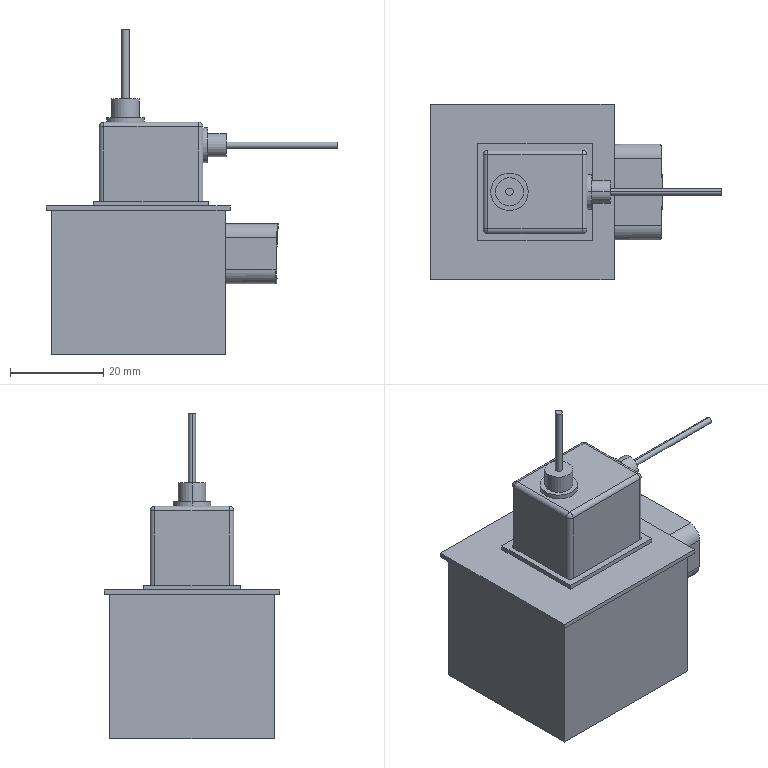Part | SolidWorks | features ICE 10, Extrusion 1, Fillet 1 | 2 solids | 70 faces | box 62.713 x 37.625 x 70 mm | volume 50756 mm3 | plane 37 | cylinder 28 | sphere 4 | spline 1 | commonest cylinder face diameters 2 x8 6 x6 4 x4 1.384 x2 1.572 x2 4.938 x2